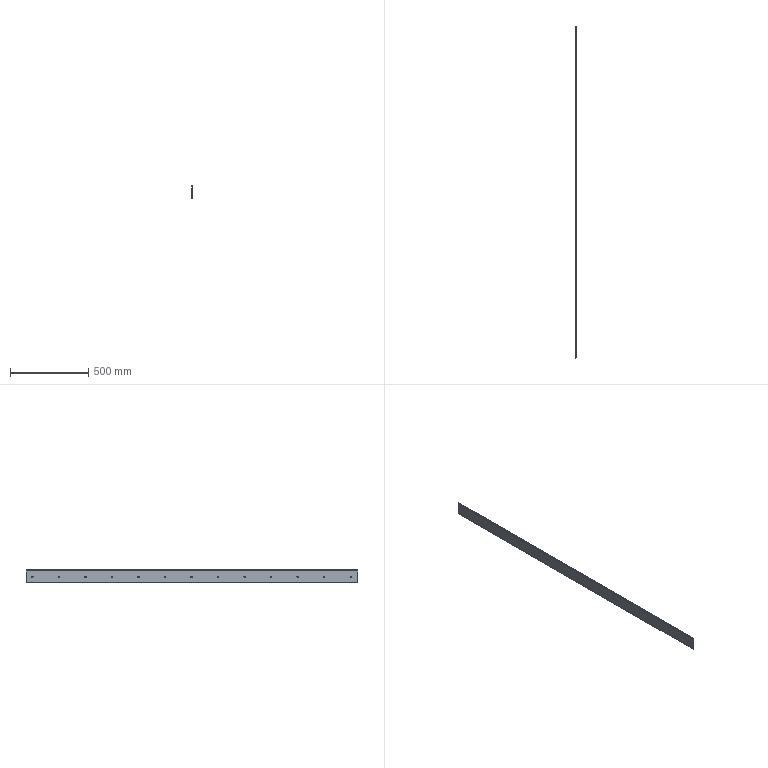Part | NX | features solid 2 | 1 solid | 59 faces | box 6 x 2128 x 85.24 mm | volume 403155 mm3 | cylinder 37 | plane 22 | commonest cylinder face diameters 8.1 x26 0.5 x10 0.6 x1